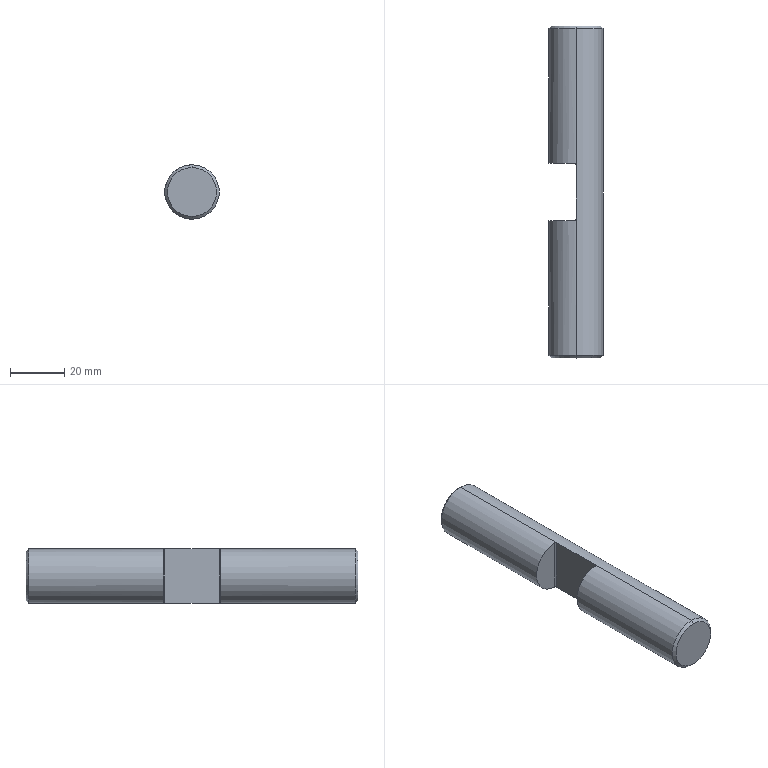Part | SolidWorks | features Chamfer 1, Cut 1, Extrusion 1 | 1 solid | 14 faces | box 20 x 122 x 20 mm | volume 34970 mm3 | cylinder 5 | plane 5 | cone 4 | commonest cylinder face diameters 20 x3 1 x2
STEP:
#1=CARTESIAN_POINT('',(0.,61.,9.));
#2=VERTEX_POINT('',#1);
#3=CARTESIAN_POINT('',(0.,61.,-9.));
#4=VERTEX_POINT('',#3);
#5=CARTESIAN_POINT('',(0.,61.,0.));
#6=DIRECTION('',(0.,1.,0.));
#7=DIRECTION('',(0.,0.,1.));
#8=AXIS2_PLACEMENT_3D('',#5,#6,#7);
#9=CIRCLE('',#8,9.);
#10=EDGE_CURVE('',#2,#4,#9,.T.);
#11=ORIENTED_EDGE('',*,*,#10,.F.);
#12=CARTESIAN_POINT('',(0.,60.,10.));
#13=VERTEX_POINT('',#12);
#14=CARTESIAN_POINT('',(0.,61.,9.));
#15=DIRECTION('',(0.,-0.7071,0.7071));
#16=VECTOR('',#15,1000.);
#17=LINE('',#14,#16);
#18=EDGE_CURVE('',#2,#13,#17,.T.);
#19=ORIENTED_EDGE('',*,*,#18,.T.);
#20=CARTESIAN_POINT('',(0.,60.,-10.));
#21=VERTEX_POINT('',#20);
#22=CARTESIAN_POINT('',(0.,60.,0.));
#23=DIRECTION('',(0.,-1.,0.));
#24=DIRECTION('',(0.,0.,1.));
#25=AXIS2_PLACEMENT_3D('',#22,#23,#24);
#26=CIRCLE('',#25,10.);
#27=EDGE_CURVE('',#21,#13,#26,.T.);
#28=ORIENTED_EDGE('',*,*,#27,.F.);
#29=CARTESIAN_POINT('',(0.,61.,-9.));
#30=DIRECTION('',(0.,-0.7071,-0.7071));
#31=VECTOR('',#30,1000.);
#32=LINE('',#29,#31);
#33=EDGE_CURVE('',#4,#21,#32,.T.);
#34=ORIENTED_EDGE('',*,*,#33,.F.);
#35=EDGE_LOOP('',(#11,#19,#28,#34));
#36=FACE_OUTER_BOUND('',#35,.T.);
#37=CARTESIAN_POINT('',(0.,61.,0.));
#38=DIRECTION('',(0.,-1.,0.));
#39=DIRECTION('',(0.,0.,-1.));
#40=AXIS2_PLACEMENT_3D('',#37,#38,#39);
#41=CONICAL_SURFACE('',#40,9.,0.7854);
#42=ADVANCED_FACE('',(#36),#41,.T.);
#43=CARTESIAN_POINT('',(0.,-61.,-9.));
#44=VERTEX_POINT('',#43);
#45=CARTESIAN_POINT('',(0.,-61.,9.));
#46=VERTEX_POINT('',#45);
#47=CARTESIAN_POINT('',(0.,-61.,0.));
#48=DIRECTION('',(0.,-1.,0.));
#49=DIRECTION('',(0.,0.,1.));
#50=AXIS2_PLACEMENT_3D('',#47,#48,#49);
#51=CIRCLE('',#50,9.);
#52=EDGE_CURVE('',#44,#46,#51,.T.);
#53=ORIENTED_EDGE('',*,*,#52,.F.);
#54=CARTESIAN_POINT('',(0.,-60.,-10.));
#55=VERTEX_POINT('',#54);
#56=CARTESIAN_POINT('',(0.,-60.,-10.));
#57=DIRECTION('',(0.,0.7071,-0.7071));
#58=VECTOR('',#57,1000.);
#59=LINE('',#56,#58);
#60=EDGE_CURVE('',#44,#55,#59,.T.);
#61=ORIENTED_EDGE('',*,*,#60,.T.);
#62=CARTESIAN_POINT('',(0.,-60.,10.));
#63=VERTEX_POINT('',#62);
#64=CARTESIAN_POINT('',(0.,-60.,0.));
#65=DIRECTION('',(0.,1.,0.));
#66=DIRECTION('',(0.,0.,1.));
#67=AXIS2_PLACEMENT_3D('',#64,#65,#66);
#68=CIRCLE('',#67,10.);
#69=EDGE_CURVE('',#63,#55,#68,.T.);
#70=ORIENTED_EDGE('',*,*,#69,.F.);
#71=CARTESIAN_POINT('',(0.,-60.,10.));
#72=DIRECTION('',(0.,0.7071,0.7071));
#73=VECTOR('',#72,1000.);
#74=LINE('',#71,#73);
#75=EDGE_CURVE('',#46,#63,#74,.T.);
#76=ORIENTED_EDGE('',*,*,#75,.F.);
#77=EDGE_LOOP('',(#53,#61,#70,#76));
#78=FACE_OUTER_BOUND('',#77,.T.);
#79=CARTESIAN_POINT('',(0.,-60.,0.));
#80=DIRECTION('',(0.,1.,0.));
#81=DIRECTION('',(0.,0.,1.));
#82=AXIS2_PLACEMENT_3D('',#79,#80,#81);
#83=CONICAL_SURFACE('',#82,10.,0.7854);
#84=ADVANCED_FACE('',(#78),#83,.T.);
#85=ORIENTED_EDGE('',*,*,#69,.T.);
#86=CARTESIAN_POINT('',(0.,-10.,-10.));
#87=VERTEX_POINT('',#86);
#88=CARTESIAN_POINT('',(0.,-61.,-10.));
#89=DIRECTION('',(0.,1.,0.));
#90=VECTOR('',#89,1000.);
#91=LINE('',#88,#90);
#92=EDGE_CURVE('',#55,#87,#91,.T.);
#93=ORIENTED_EDGE('',*,*,#92,.T.);
#94=CARTESIAN_POINT('',(0.,10.,-10.));
#95=VERTEX_POINT('',#94);
#96=CARTESIAN_POINT('',(0.,-61.,-10.));
#97=DIRECTION('',(0.,1.,0.));
#98=VECTOR('',#97,1000.);
#99=LINE('',#96,#98);
#100=EDGE_CURVE('',#87,#95,#99,.T.);
#101=ORIENTED_EDGE('',*,*,#100,.T.);
#102=CARTESIAN_POINT('',(0.,-61.,-10.));
#103=DIRECTION('',(0.,1.,0.));
#104=VECTOR('',#103,1000.);
#105=LINE('',#102,#104);
#106=EDGE_CURVE('',#95,#21,#105,.T.);
#107=ORIENTED_EDGE('',*,*,#106,.T.);
#108=ORIENTED_EDGE('',*,*,#27,.T.);
#109=CARTESIAN_POINT('',(0.,10.,10.));
#110=VERTEX_POINT('',#109);
#111=CARTESIAN_POINT('',(0.,-61.,10.));
#112=DIRECTION('',(0.,1.,0.));
#113=VECTOR('',#112,1000.);
#114=LINE('',#111,#113);
#115=EDGE_CURVE('',#110,#13,#114,.T.);
#116=ORIENTED_EDGE('',*,*,#115,.F.);
#117=CARTESIAN_POINT('',(0.,-10.,10.));
#118=VERTEX_POINT('',#117);
#119=CARTESIAN_POINT('',(0.,-61.,10.));
#120=DIRECTION('',(0.,1.,0.));
#121=VECTOR('',#120,1000.);
#122=LINE('',#119,#121);
#123=EDGE_CURVE('',#118,#110,#122,.T.);
#124=ORIENTED_EDGE('',*,*,#123,.F.);
#125=CARTESIAN_POINT('',(0.,-61.,10.));
#126=DIRECTION('',(0.,1.,0.));
#127=VECTOR('',#126,1000.);
#128=LINE('',#125,#127);
#129=EDGE_CURVE('',#63,#118,#128,.T.);
#130=ORIENTED_EDGE('',*,*,#129,.F.);
#131=EDGE_LOOP('',(#85,#93,#101,#107,#108,#116,#124,#130));
#132=FACE_OUTER_BOUND('',#131,.T.);
#133=CARTESIAN_POINT('',(0.,-61.,0.));
#134=DIRECTION('',(0.,1.,0.));
#135=DIRECTION('',(0.,0.,1.));
#136=AXIS2_PLACEMENT_3D('',#133,#134,#135);
#137=CYLINDRICAL_SURFACE('',#136,10.);
#138=ADVANCED_FACE('',(#132),#137,.T.);
#139=ORIENTED_EDGE('',*,*,#92,.F.);
#140=CARTESIAN_POINT('',(0.,-60.,0.));
#141=DIRECTION('',(0.,1.,0.));
#142=DIRECTION('',(0.,0.,1.));
#143=AXIS2_PLACEMENT_3D('',#140,#141,#142);
#144=CIRCLE('',#143,10.);
#145=EDGE_CURVE('',#55,#63,#144,.T.);
#146=ORIENTED_EDGE('',*,*,#145,.T.);
#147=ORIENTED_EDGE('',*,*,#129,.T.);
#148=CARTESIAN_POINT('',(-0.5,-10.5,9.987));
#149=VERTEX_POINT('',#148);
#150=CARTESIAN_POINT('',(-0.5,-10.5,9.987));
#151=CARTESIAN_POINT('',(-0.3681,-10.5,9.994));
#152=CARTESIAN_POINT('',(-0.2389,-10.446,9.998));
#153=CARTESIAN_POINT('',(-0.05437,-10.262,10.));
#154=CARTESIAN_POINT('',(0.,-10.132,10.));
#155=CARTESIAN_POINT('',(0.,-10.,10.));
#156=B_SPLINE_CURVE_WITH_KNOTS('',3,(#150,#151,#152,#153,#154,#155),.UNSPECIFIED.,.F.,.F.,(4,2,4),(0.,0.0003906,0.0007813),.UNSPECIFIED.);
#157=EDGE_CURVE('',#149,#118,#156,.T.);
#158=ORIENTED_EDGE('',*,*,#157,.F.);
#159=CARTESIAN_POINT('',(-0.5,-10.5,-9.987));
#160=VERTEX_POINT('',#159);
#161=CARTESIAN_POINT('',(0.,-10.5,0.));
#162=DIRECTION('',(0.,1.,0.));
#163=DIRECTION('',(-1.,0.,0.));
#164=AXIS2_PLACEMENT_3D('',#161,#162,#163);
#165=CIRCLE('',#164,10.);
#166=EDGE_CURVE('',#160,#149,#165,.T.);
#167=ORIENTED_EDGE('',*,*,#166,.F.);
#168=CARTESIAN_POINT('',(-0.5,-10.5,-9.987));
#169=CARTESIAN_POINT('',(-0.3681,-10.5,-9.994));
#170=CARTESIAN_POINT('',(-0.2389,-10.446,-9.998));
#171=CARTESIAN_POINT('',(-0.05437,-10.262,-10.));
#172=CARTESIAN_POINT('',(0.,-10.132,-10.));
#173=CARTESIAN_POINT('',(0.,-10.,-10.));
#174=B_SPLINE_CURVE_WITH_KNOTS('',3,(#168,#169,#170,#171,#172,#173),.UNSPECIFIED.,.F.,.F.,(4,2,4),(0.,0.0003906,0.0007813),.UNSPECIFIED.);
#175=EDGE_CURVE('',#160,#87,#174,.T.);
#176=ORIENTED_EDGE('',*,*,#175,.T.);
#177=EDGE_LOOP('',(#139,#146,#147,#158,#167,#176));
#178=FACE_OUTER_BOUND('',#177,.T.);
#179=CARTESIAN_POINT('',(0.,-61.,0.));
#180=DIRECTION('',(0.,1.,0.));
#181=DIRECTION('',(0.,0.,1.));
#182=AXIS2_PLACEMENT_3D('',#179,#180,#181);
#183=CYLINDRICAL_SURFACE('',#182,10.);
#184=ADVANCED_FACE('',(#178),#183,.T.);
#185=ORIENTED_EDGE('',*,*,#106,.F.);
#186=CARTESIAN_POINT('',(-0.5,10.5,-9.987));
#187=VERTEX_POINT('',#186);
#188=CARTESIAN_POINT('',(0.,10.,-10.));
#189=CARTESIAN_POINT('',(0.,10.132,-10.));
#190=CARTESIAN_POINT('',(-0.05418,10.261,-10.));
#191=CARTESIAN_POINT('',(-0.2386,10.446,-9.998));
#192=CARTESIAN_POINT('',(-0.3681,10.5,-9.994));
#193=CARTESIAN_POINT('',(-0.5,10.5,-9.987));
#194=B_SPLINE_CURVE_WITH_KNOTS('',3,(#188,#189,#190,#191,#192,#193),.UNSPECIFIED.,.F.,.F.,(4,2,4),(0.,0.0003906,0.0007813),.UNSPECIFIED.);
#195=EDGE_CURVE('',#95,#187,#194,.T.);
#196=ORIENTED_EDGE('',*,*,#195,.T.);
#197=CARTESIAN_POINT('',(-0.5,10.5,9.987));
#198=VERTEX_POINT('',#197);
#199=CARTESIAN_POINT('',(0.,10.5,0.));
#200=DIRECTION('',(0.,-1.,0.));
#201=DIRECTION('',(1.,0.,0.));
#202=AXIS2_PLACEMENT_3D('',#199,#200,#201);
#203=CIRCLE('',#202,10.);
#204=EDGE_CURVE('',#198,#187,#203,.T.);
#205=ORIENTED_EDGE('',*,*,#204,.F.);
#206=CARTESIAN_POINT('',(0.,10.,10.));
#207=CARTESIAN_POINT('',(0.,10.132,10.));
#208=CARTESIAN_POINT('',(-0.05418,10.261,10.));
#209=CARTESIAN_POINT('',(-0.2386,10.446,9.998));
#210=CARTESIAN_POINT('',(-0.3681,10.5,9.994));
#211=CARTESIAN_POINT('',(-0.5,10.5,9.987));
#212=B_SPLINE_CURVE_WITH_KNOTS('',3,(#206,#207,#208,#209,#210,#211),.UNSPECIFIED.,.F.,.F.,(4,2,4),(0.,0.0003906,0.0007813),.UNSPECIFIED.);
#213=EDGE_CURVE('',#110,#198,#212,.T.);
#214=ORIENTED_EDGE('',*,*,#213,.F.);
#215=ORIENTED_EDGE('',*,*,#115,.T.);
#216=CARTESIAN_POINT('',(0.,60.,0.));
#217=DIRECTION('',(0.,-1.,0.));
#218=DIRECTION('',(0.,0.,1.));
#219=AXIS2_PLACEMENT_3D('',#216,#217,#218);
#220=CIRCLE('',#219,10.);
#221=EDGE_CURVE('',#13,#21,#220,.T.);
#222=ORIENTED_EDGE('',*,*,#221,.T.);
#223=EDGE_LOOP('',(#185,#196,#205,#214,#215,#222));
#224=FACE_OUTER_BOUND('',#223,.T.);
#225=CARTESIAN_POINT('',(0.,-61.,0.));
#226=DIRECTION('',(0.,1.,0.));
#227=DIRECTION('',(0.,0.,1.));
#228=AXIS2_PLACEMENT_3D('',#225,#226,#227);
#229=CYLINDRICAL_SURFACE('',#228,10.);
#230=ADVANCED_FACE('',(#224),#229,.T.);
#231=CARTESIAN_POINT('',(0.,-61.,0.));
#232=DIRECTION('',(0.,-1.,0.));
#233=DIRECTION('',(0.,0.,1.));
#234=AXIS2_PLACEMENT_3D('',#231,#232,#233);
#235=CIRCLE('',#234,9.);
#236=EDGE_CURVE('',#46,#44,#235,.T.);
#237=ORIENTED_EDGE('',*,*,#236,.T.);
#238=ORIENTED_EDGE('',*,*,#52,.T.);
#239=EDGE_LOOP('',(#237,#238));
#240=FACE_OUTER_BOUND('',#239,.T.);
#241=CARTESIAN_POINT('',(0.,-61.,0.));
#242=DIRECTION('',(0.,1.,0.));
#243=DIRECTION('',(0.,0.,1.));
#244=AXIS2_PLACEMENT_3D('',#241,#242,#243);
#245=PLANE('',#244);
#246=ADVANCED_FACE('',(#240),#245,.F.);
#247=CARTESIAN_POINT('',(0.,61.,0.));
#248=DIRECTION('',(0.,1.,0.));
#249=DIRECTION('',(0.,0.,1.));
#250=AXIS2_PLACEMENT_3D('',#247,#248,#249);
#251=CIRCLE('',#250,9.);
#252=EDGE_CURVE('',#4,#2,#251,.T.);
#253=ORIENTED_EDGE('',*,*,#252,.T.);
#254=ORIENTED_EDGE('',*,*,#10,.T.);
#255=EDGE_LOOP('',(#253,#254));
#256=FACE_OUTER_BOUND('',#255,.T.);
#257=CARTESIAN_POINT('',(0.,61.,0.));
#258=DIRECTION('',(0.,1.,0.));
#259=DIRECTION('',(0.,0.,1.));
#260=AXIS2_PLACEMENT_3D('',#257,#258,#259);
#261=PLANE('',#260);
#262=ADVANCED_FACE('',(#256),#261,.T.);
#263=ORIENTED_EDGE('',*,*,#204,.T.);
#264=CARTESIAN_POINT('',(-0.5,10.5,10.001));
#265=DIRECTION('',(0.,0.,-1.));
#266=VECTOR('',#265,1000.);
#267=LINE('',#264,#266);
#268=EDGE_CURVE('',#198,#187,#267,.T.);
#269=ORIENTED_EDGE('',*,*,#268,.F.);
#270=EDGE_LOOP('',(#263,#269));
#271=FACE_OUTER_BOUND('',#270,.T.);
#272=CARTESIAN_POINT('',(-0.5,10.5,10.001));
#273=DIRECTION('',(0.,-1.,0.));
#274=DIRECTION('',(1.,0.,0.));
#275=AXIS2_PLACEMENT_3D('',#272,#273,#274);
#276=PLANE('',#275);
#277=ADVANCED_FACE('',(#271),#276,.T.);
#278=ORIENTED_EDGE('',*,*,#166,.T.);
#279=CARTESIAN_POINT('',(-0.5,-10.5,10.001));
#280=DIRECTION('',(0.,0.,-1.));
#281=VECTOR('',#280,1000.);
#282=LINE('',#279,#281);
#283=EDGE_CURVE('',#149,#160,#282,.T.);
#284=ORIENTED_EDGE('',*,*,#283,.T.);
#285=EDGE_LOOP('',(#278,#284));
#286=FACE_OUTER_BOUND('',#285,.T.);
#287=CARTESIAN_POINT('',(-0.5,-10.5,10.001));
#288=DIRECTION('',(0.,1.,0.));
#289=DIRECTION('',(-1.,0.,0.));
#290=AXIS2_PLACEMENT_3D('',#287,#288,#289);
#291=PLANE('',#290);
#292=ADVANCED_FACE('',(#286),#291,.T.);
#293=ORIENTED_EDGE('',*,*,#213,.T.);
#294=ORIENTED_EDGE('',*,*,#268,.T.);
#295=ORIENTED_EDGE('',*,*,#195,.F.);
#296=CARTESIAN_POINT('',(0.,10.,10.001));
#297=DIRECTION('',(0.,0.,-1.));
#298=VECTOR('',#297,1000.);
#299=LINE('',#296,#298);
#300=EDGE_CURVE('',#110,#95,#299,.T.);
#301=ORIENTED_EDGE('',*,*,#300,.F.);
#302=EDGE_LOOP('',(#293,#294,#295,#301));
#303=FACE_OUTER_BOUND('',#302,.T.);
#304=CARTESIAN_POINT('',(-0.5,10.,10.001));
#305=DIRECTION('',(0.,0.,-1.));
#306=DIRECTION('',(-1.,0.,0.));
#307=AXIS2_PLACEMENT_3D('',#304,#305,#306);
#308=CYLINDRICAL_SURFACE('',#307,0.5);
#309=ADVANCED_FACE('',(#303),#308,.F.);
#310=ORIENTED_EDGE('',*,*,#157,.T.);
#311=CARTESIAN_POINT('',(0.,-10.,10.001));
#312=DIRECTION('',(0.,0.,-1.));
#313=VECTOR('',#312,1000.);
#314=LINE('',#311,#313);
#315=EDGE_CURVE('',#118,#87,#314,.T.);
#316=ORIENTED_EDGE('',*,*,#315,.T.);
#317=ORIENTED_EDGE('',*,*,#175,.F.);
#318=ORIENTED_EDGE('',*,*,#283,.F.);
#319=EDGE_LOOP('',(#310,#316,#317,#318));
#320=FACE_OUTER_BOUND('',#319,.T.);
#321=CARTESIAN_POINT('',(-0.5,-10.,10.001));
#322=DIRECTION('',(0.,0.,-1.));
#323=DIRECTION('',(-1.,0.,0.));
#324=AXIS2_PLACEMENT_3D('',#321,#322,#323);
#325=CYLINDRICAL_SURFACE('',#324,0.5);
#326=ADVANCED_FACE('',(#320),#325,.F.);
#327=ORIENTED_EDGE('',*,*,#123,.T.);
#328=ORIENTED_EDGE('',*,*,#300,.T.);
#329=ORIENTED_EDGE('',*,*,#100,.F.);
#330=ORIENTED_EDGE('',*,*,#315,.F.);
#331=EDGE_LOOP('',(#327,#328,#329,#330));
#332=FACE_OUTER_BOUND('',#331,.T.);
#333=CARTESIAN_POINT('',(0.,-10.,10.001));
#334=DIRECTION('',(-1.,0.,0.));
#335=DIRECTION('',(0.,-1.,0.));
#336=AXIS2_PLACEMENT_3D('',#333,#334,#335);
#337=PLANE('',#336);
#338=ADVANCED_FACE('',(#332),#337,.T.);
#339=ORIENTED_EDGE('',*,*,#60,.F.);
#340=ORIENTED_EDGE('',*,*,#236,.F.);
#341=ORIENTED_EDGE('',*,*,#75,.T.);
#342=ORIENTED_EDGE('',*,*,#145,.F.);
#343=EDGE_LOOP('',(#339,#340,#341,#342));
#344=FACE_OUTER_BOUND('',#343,.T.);
#345=CARTESIAN_POINT('',(0.,-60.,0.));
#346=DIRECTION('',(0.,1.,0.));
#347=DIRECTION('',(0.,0.,1.));
#348=AXIS2_PLACEMENT_3D('',#345,#346,#347);
#349=CONICAL_SURFACE('',#348,10.,0.7854);
#350=ADVANCED_FACE('',(#344),#349,.T.);
#351=ORIENTED_EDGE('',*,*,#18,.F.);
#352=ORIENTED_EDGE('',*,*,#252,.F.);
#353=ORIENTED_EDGE('',*,*,#33,.T.);
#354=ORIENTED_EDGE('',*,*,#221,.F.);
#355=EDGE_LOOP('',(#351,#352,#353,#354));
#356=FACE_OUTER_BOUND('',#355,.T.);
#357=CARTESIAN_POINT('',(0.,61.,0.));
#358=DIRECTION('',(0.,-1.,0.));
#359=DIRECTION('',(0.,0.,-1.));
#360=AXIS2_PLACEMENT_3D('',#357,#358,#359);
#361=CONICAL_SURFACE('',#360,9.,0.7854);
#362=ADVANCED_FACE('',(#356),#361,.T.);
#363=CLOSED_SHELL('',(#42,#84,#138,#184,#230,#246,#262,#277,#292,#309,#326,#338,#350,#362));
#364=MANIFOLD_SOLID_BREP('',#363);
#365=CARTESIAN_POINT('',(0.,0.,0.));
#366=DIRECTION('',(0.,0.,1.));
#367=DIRECTION('',(1.,0.,0.));
#368=AXIS2_PLACEMENT_3D('',#365,#366,#367);
#369=(LENGTH_UNIT()NAMED_UNIT(*)SI_UNIT(.MILLI.,.METRE.));
#370=UNCERTAINTY_MEASURE_WITH_UNIT(LENGTH_MEASURE(0.00001),#369,'','');
#371=(NAMED_UNIT(*)PLANE_ANGLE_UNIT()SI_UNIT($,.RADIAN.));
#372=(NAMED_UNIT(*)SI_UNIT($,.STERADIAN.)SOLID_ANGLE_UNIT());
#373=(GEOMETRIC_REPRESENTATION_CONTEXT(3)GLOBAL_UNCERTAINTY_ASSIGNED_CONTEXT((#370))GLOBAL_UNIT_ASSIGNED_CONTEXT((#369,#371,#372))REPRESENTATION_CONTEXT('',''));
#374=ADVANCED_BREP_SHAPE_REPRESENTATION('',(#364,#368),#373);